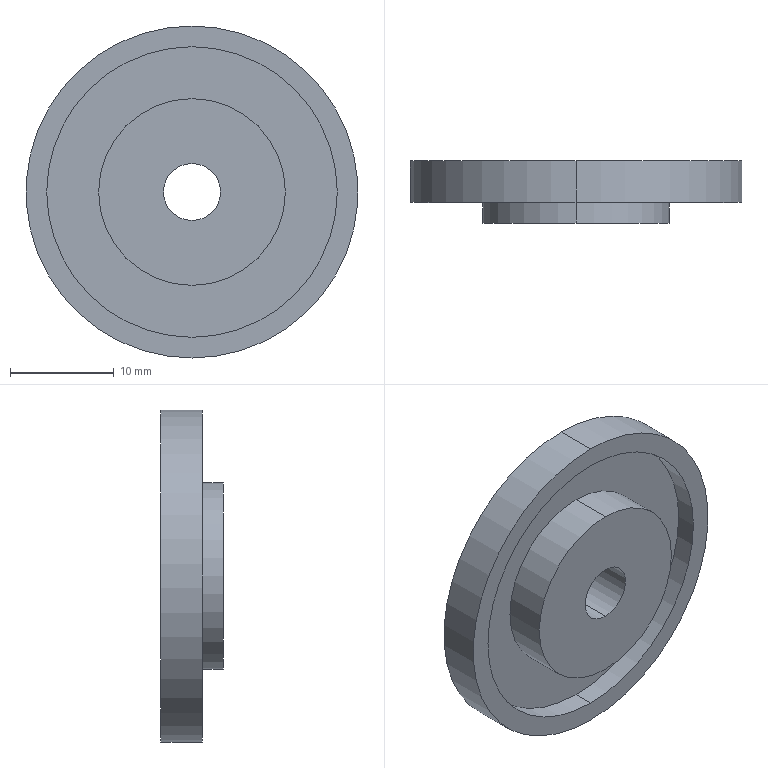Part | SolidWorks | features Revolution 1 | 1 solid | 14 faces | box 32 x 6 x 32 mm | volume 2776 mm3 | cylinder 8 | plane 4 | cone 2 | commonest cylinder face diameters 5.5 x2 18 x2 28 x2 32 x2
STEP:
#1=CARTESIAN_POINT('',(0.,-0.2262,-14.));
#2=VERTEX_POINT('',#1);
#3=CARTESIAN_POINT('',(0.,-0.2262,14.));
#4=VERTEX_POINT('',#3);
#5=CARTESIAN_POINT('',(0.,-0.2262,0.));
#6=DIRECTION('',(0.,1.,0.));
#7=DIRECTION('',(0.,0.,1.));
#8=AXIS2_PLACEMENT_3D('',#5,#6,#7);
#9=CIRCLE('',#8,14.);
#10=EDGE_CURVE('',#2,#4,#9,.T.);
#11=ORIENTED_EDGE('',*,*,#10,.F.);
#12=CARTESIAN_POINT('',(0.,1.774,-14.));
#13=VERTEX_POINT('',#12);
#14=CARTESIAN_POINT('',(0.,9.909,-14.));
#15=DIRECTION('',(0.,1.,0.));
#16=VECTOR('',#15,1000.);
#17=LINE('',#14,#16);
#18=EDGE_CURVE('',#2,#13,#17,.T.);
#19=ORIENTED_EDGE('',*,*,#18,.T.);
#20=CARTESIAN_POINT('',(0.,1.774,14.));
#21=VERTEX_POINT('',#20);
#22=CARTESIAN_POINT('',(0.,1.774,0.));
#23=DIRECTION('',(0.,1.,0.));
#24=DIRECTION('',(0.,0.,1.));
#25=AXIS2_PLACEMENT_3D('',#22,#23,#24);
#26=CIRCLE('',#25,14.);
#27=EDGE_CURVE('',#13,#21,#26,.T.);
#28=ORIENTED_EDGE('',*,*,#27,.T.);
#29=CARTESIAN_POINT('',(0.,9.909,14.));
#30=DIRECTION('',(0.,1.,0.));
#31=VECTOR('',#30,1000.);
#32=LINE('',#29,#31);
#33=EDGE_CURVE('',#4,#21,#32,.T.);
#34=ORIENTED_EDGE('',*,*,#33,.F.);
#35=EDGE_LOOP('',(#11,#19,#28,#34));
#36=FACE_OUTER_BOUND('',#35,.T.);
#37=CARTESIAN_POINT('',(0.,9.909,0.));
#38=DIRECTION('',(0.,1.,0.));
#39=DIRECTION('',(0.,0.,1.));
#40=AXIS2_PLACEMENT_3D('',#37,#38,#39);
#41=CYLINDRICAL_SURFACE('',#40,14.);
#42=ADVANCED_FACE('',(#36),#41,.F.);
#43=CARTESIAN_POINT('',(0.,-0.2262,16.));
#44=VERTEX_POINT('',#43);
#45=CARTESIAN_POINT('',(0.,-0.2262,-16.));
#46=VERTEX_POINT('',#45);
#47=CARTESIAN_POINT('',(0.,-0.2262,0.));
#48=DIRECTION('',(0.,1.,0.));
#49=DIRECTION('',(0.,0.,1.));
#50=AXIS2_PLACEMENT_3D('',#47,#48,#49);
#51=CIRCLE('',#50,16.);
#52=EDGE_CURVE('',#44,#46,#51,.T.);
#53=ORIENTED_EDGE('',*,*,#52,.T.);
#54=CARTESIAN_POINT('',(0.,3.774,-16.));
#55=VERTEX_POINT('',#54);
#56=CARTESIAN_POINT('',(0.,9.909,-16.));
#57=DIRECTION('',(0.,1.,0.));
#58=VECTOR('',#57,1000.);
#59=LINE('',#56,#58);
#60=EDGE_CURVE('',#46,#55,#59,.T.);
#61=ORIENTED_EDGE('',*,*,#60,.T.);
#62=CARTESIAN_POINT('',(0.,3.774,16.));
#63=VERTEX_POINT('',#62);
#64=CARTESIAN_POINT('',(0.,3.774,0.));
#65=DIRECTION('',(0.,1.,0.));
#66=DIRECTION('',(0.,0.,1.));
#67=AXIS2_PLACEMENT_3D('',#64,#65,#66);
#68=CIRCLE('',#67,16.);
#69=EDGE_CURVE('',#63,#55,#68,.T.);
#70=ORIENTED_EDGE('',*,*,#69,.F.);
#71=CARTESIAN_POINT('',(0.,9.909,16.));
#72=DIRECTION('',(0.,1.,0.));
#73=VECTOR('',#72,1000.);
#74=LINE('',#71,#73);
#75=EDGE_CURVE('',#44,#63,#74,.T.);
#76=ORIENTED_EDGE('',*,*,#75,.F.);
#77=EDGE_LOOP('',(#53,#61,#70,#76));
#78=FACE_OUTER_BOUND('',#77,.T.);
#79=CARTESIAN_POINT('',(0.,9.909,0.));
#80=DIRECTION('',(0.,1.,0.));
#81=DIRECTION('',(0.,0.,1.));
#82=AXIS2_PLACEMENT_3D('',#79,#80,#81);
#83=CYLINDRICAL_SURFACE('',#82,16.);
#84=ADVANCED_FACE('',(#78),#83,.T.);
#85=CARTESIAN_POINT('',(0.,1.774,-2.75));
#86=VERTEX_POINT('',#85);
#87=CARTESIAN_POINT('',(0.,1.774,2.75));
#88=VERTEX_POINT('',#87);
#89=CARTESIAN_POINT('',(0.,1.774,0.));
#90=DIRECTION('',(0.,1.,0.));
#91=DIRECTION('',(0.,0.,1.));
#92=AXIS2_PLACEMENT_3D('',#89,#90,#91);
#93=CIRCLE('',#92,2.75);
#94=EDGE_CURVE('',#86,#88,#93,.T.);
#95=ORIENTED_EDGE('',*,*,#94,.F.);
#96=CARTESIAN_POINT('',(0.,3.774,-6.214));
#97=VERTEX_POINT('',#96);
#98=CARTESIAN_POINT('',(0.,1.774,-2.75));
#99=DIRECTION('',(0.,0.5,-0.866));
#100=VECTOR('',#99,1000.);
#101=LINE('',#98,#100);
#102=EDGE_CURVE('',#86,#97,#101,.T.);
#103=ORIENTED_EDGE('',*,*,#102,.T.);
#104=CARTESIAN_POINT('',(0.,3.774,6.214));
#105=VERTEX_POINT('',#104);
#106=CARTESIAN_POINT('',(0.,3.774,0.));
#107=DIRECTION('',(0.,1.,0.));
#108=DIRECTION('',(0.,0.,1.));
#109=AXIS2_PLACEMENT_3D('',#106,#107,#108);
#110=CIRCLE('',#109,6.214);
#111=EDGE_CURVE('',#97,#105,#110,.T.);
#112=ORIENTED_EDGE('',*,*,#111,.T.);
#113=CARTESIAN_POINT('',(0.,1.774,2.75));
#114=DIRECTION('',(0.,0.5,0.866));
#115=VECTOR('',#114,1000.);
#116=LINE('',#113,#115);
#117=EDGE_CURVE('',#88,#105,#116,.T.);
#118=ORIENTED_EDGE('',*,*,#117,.F.);
#119=EDGE_LOOP('',(#95,#103,#112,#118));
#120=FACE_OUTER_BOUND('',#119,.T.);
#121=CARTESIAN_POINT('',(0.,1.774,0.));
#122=DIRECTION('',(0.,1.,0.));
#123=DIRECTION('',(0.,0.,1.));
#124=AXIS2_PLACEMENT_3D('',#121,#122,#123);
#125=CONICAL_SURFACE('',#124,2.75,1.047);
#126=ADVANCED_FACE('',(#120),#125,.F.);
#127=CARTESIAN_POINT('',(0.,-2.226,-2.75));
#128=VERTEX_POINT('',#127);
#129=CARTESIAN_POINT('',(0.,-2.226,2.75));
#130=VERTEX_POINT('',#129);
#131=CARTESIAN_POINT('',(0.,-2.226,0.));
#132=DIRECTION('',(0.,1.,0.));
#133=DIRECTION('',(0.,0.,1.));
#134=AXIS2_PLACEMENT_3D('',#131,#132,#133);
#135=CIRCLE('',#134,2.75);
#136=EDGE_CURVE('',#128,#130,#135,.T.);
#137=ORIENTED_EDGE('',*,*,#136,.F.);
#138=CARTESIAN_POINT('',(0.,9.909,-2.75));
#139=DIRECTION('',(0.,1.,0.));
#140=VECTOR('',#139,1000.);
#141=LINE('',#138,#140);
#142=EDGE_CURVE('',#128,#86,#141,.T.);
#143=ORIENTED_EDGE('',*,*,#142,.T.);
#144=ORIENTED_EDGE('',*,*,#94,.T.);
#145=CARTESIAN_POINT('',(0.,9.909,2.75));
#146=DIRECTION('',(0.,1.,0.));
#147=VECTOR('',#146,1000.);
#148=LINE('',#145,#147);
#149=EDGE_CURVE('',#130,#88,#148,.T.);
#150=ORIENTED_EDGE('',*,*,#149,.F.);
#151=EDGE_LOOP('',(#137,#143,#144,#150));
#152=FACE_OUTER_BOUND('',#151,.T.);
#153=CARTESIAN_POINT('',(0.,9.909,0.));
#154=DIRECTION('',(0.,1.,0.));
#155=DIRECTION('',(0.,0.,1.));
#156=AXIS2_PLACEMENT_3D('',#153,#154,#155);
#157=CYLINDRICAL_SURFACE('',#156,2.75);
#158=ADVANCED_FACE('',(#152),#157,.F.);
#159=CARTESIAN_POINT('',(0.,-2.226,9.));
#160=VERTEX_POINT('',#159);
#161=CARTESIAN_POINT('',(0.,-2.226,-9.));
#162=VERTEX_POINT('',#161);
#163=CARTESIAN_POINT('',(0.,-2.226,0.));
#164=DIRECTION('',(0.,1.,0.));
#165=DIRECTION('',(0.,0.,1.));
#166=AXIS2_PLACEMENT_3D('',#163,#164,#165);
#167=CIRCLE('',#166,9.);
#168=EDGE_CURVE('',#160,#162,#167,.T.);
#169=ORIENTED_EDGE('',*,*,#168,.T.);
#170=CARTESIAN_POINT('',(0.,1.774,-9.));
#171=VERTEX_POINT('',#170);
#172=CARTESIAN_POINT('',(0.,9.909,-9.));
#173=DIRECTION('',(0.,1.,0.));
#174=VECTOR('',#173,1000.);
#175=LINE('',#172,#174);
#176=EDGE_CURVE('',#162,#171,#175,.T.);
#177=ORIENTED_EDGE('',*,*,#176,.T.);
#178=CARTESIAN_POINT('',(0.,1.774,9.));
#179=VERTEX_POINT('',#178);
#180=CARTESIAN_POINT('',(0.,1.774,0.));
#181=DIRECTION('',(0.,1.,0.));
#182=DIRECTION('',(0.,0.,1.));
#183=AXIS2_PLACEMENT_3D('',#180,#181,#182);
#184=CIRCLE('',#183,9.);
#185=EDGE_CURVE('',#179,#171,#184,.T.);
#186=ORIENTED_EDGE('',*,*,#185,.F.);
#187=CARTESIAN_POINT('',(0.,9.909,9.));
#188=DIRECTION('',(0.,1.,0.));
#189=VECTOR('',#188,1000.);
#190=LINE('',#187,#189);
#191=EDGE_CURVE('',#160,#179,#190,.T.);
#192=ORIENTED_EDGE('',*,*,#191,.F.);
#193=EDGE_LOOP('',(#169,#177,#186,#192));
#194=FACE_OUTER_BOUND('',#193,.T.);
#195=CARTESIAN_POINT('',(0.,9.909,0.));
#196=DIRECTION('',(0.,1.,0.));
#197=DIRECTION('',(0.,0.,1.));
#198=AXIS2_PLACEMENT_3D('',#195,#196,#197);
#199=CYLINDRICAL_SURFACE('',#198,9.);
#200=ADVANCED_FACE('',(#194),#199,.T.);
#201=ORIENTED_EDGE('',*,*,#176,.F.);
#202=CARTESIAN_POINT('',(0.,-2.226,0.));
#203=DIRECTION('',(0.,1.,0.));
#204=DIRECTION('',(0.,0.,1.));
#205=AXIS2_PLACEMENT_3D('',#202,#203,#204);
#206=CIRCLE('',#205,9.);
#207=EDGE_CURVE('',#162,#160,#206,.T.);
#208=ORIENTED_EDGE('',*,*,#207,.T.);
#209=ORIENTED_EDGE('',*,*,#191,.T.);
#210=CARTESIAN_POINT('',(0.,1.774,0.));
#211=DIRECTION('',(0.,1.,0.));
#212=DIRECTION('',(0.,0.,1.));
#213=AXIS2_PLACEMENT_3D('',#210,#211,#212);
#214=CIRCLE('',#213,9.);
#215=EDGE_CURVE('',#171,#179,#214,.T.);
#216=ORIENTED_EDGE('',*,*,#215,.F.);
#217=EDGE_LOOP('',(#201,#208,#209,#216));
#218=FACE_OUTER_BOUND('',#217,.T.);
#219=CARTESIAN_POINT('',(0.,9.909,0.));
#220=DIRECTION('',(0.,1.,0.));
#221=DIRECTION('',(0.,0.,1.));
#222=AXIS2_PLACEMENT_3D('',#219,#220,#221);
#223=CYLINDRICAL_SURFACE('',#222,9.);
#224=ADVANCED_FACE('',(#218),#223,.T.);
#225=CARTESIAN_POINT('',(0.,-2.226,0.));
#226=DIRECTION('',(0.,1.,0.));
#227=DIRECTION('',(0.,0.,1.));
#228=AXIS2_PLACEMENT_3D('',#225,#226,#227);
#229=CIRCLE('',#228,2.75);
#230=EDGE_CURVE('',#130,#128,#229,.T.);
#231=ORIENTED_EDGE('',*,*,#230,.T.);
#232=ORIENTED_EDGE('',*,*,#136,.T.);
#233=EDGE_LOOP('',(#231,#232));
#234=FACE_BOUND('',#233,.T.);
#235=ORIENTED_EDGE('',*,*,#168,.F.);
#236=ORIENTED_EDGE('',*,*,#207,.F.);
#237=EDGE_LOOP('',(#235,#236));
#238=FACE_OUTER_BOUND('',#237,.T.);
#239=CARTESIAN_POINT('',(-2.75,-2.226,0.));
#240=DIRECTION('',(0.,-1.,0.));
#241=DIRECTION('',(0.,0.,-1.));
#242=AXIS2_PLACEMENT_3D('',#239,#240,#241);
#243=PLANE('',#242);
#244=ADVANCED_FACE('',(#234,#238),#243,.T.);
#245=ORIENTED_EDGE('',*,*,#142,.F.);
#246=ORIENTED_EDGE('',*,*,#230,.F.);
#247=ORIENTED_EDGE('',*,*,#149,.T.);
#248=CARTESIAN_POINT('',(0.,1.774,0.));
#249=DIRECTION('',(0.,1.,0.));
#250=DIRECTION('',(0.,0.,1.));
#251=AXIS2_PLACEMENT_3D('',#248,#249,#250);
#252=CIRCLE('',#251,2.75);
#253=EDGE_CURVE('',#88,#86,#252,.T.);
#254=ORIENTED_EDGE('',*,*,#253,.T.);
#255=EDGE_LOOP('',(#245,#246,#247,#254));
#256=FACE_OUTER_BOUND('',#255,.T.);
#257=CARTESIAN_POINT('',(0.,9.909,0.));
#258=DIRECTION('',(0.,1.,0.));
#259=DIRECTION('',(0.,0.,1.));
#260=AXIS2_PLACEMENT_3D('',#257,#258,#259);
#261=CYLINDRICAL_SURFACE('',#260,2.75);
#262=ADVANCED_FACE('',(#256),#261,.F.);
#263=ORIENTED_EDGE('',*,*,#102,.F.);
#264=ORIENTED_EDGE('',*,*,#253,.F.);
#265=ORIENTED_EDGE('',*,*,#117,.T.);
#266=CARTESIAN_POINT('',(0.,3.774,0.));
#267=DIRECTION('',(0.,1.,0.));
#268=DIRECTION('',(0.,0.,1.));
#269=AXIS2_PLACEMENT_3D('',#266,#267,#268);
#270=CIRCLE('',#269,6.214);
#271=EDGE_CURVE('',#105,#97,#270,.T.);
#272=ORIENTED_EDGE('',*,*,#271,.T.);
#273=EDGE_LOOP('',(#263,#264,#265,#272));
#274=FACE_OUTER_BOUND('',#273,.T.);
#275=CARTESIAN_POINT('',(0.,1.774,0.));
#276=DIRECTION('',(0.,1.,0.));
#277=DIRECTION('',(0.,0.,1.));
#278=AXIS2_PLACEMENT_3D('',#275,#276,#277);
#279=CONICAL_SURFACE('',#278,2.75,1.047);
#280=ADVANCED_FACE('',(#274),#279,.F.);
#281=ORIENTED_EDGE('',*,*,#69,.T.);
#282=CARTESIAN_POINT('',(0.,3.774,0.));
#283=DIRECTION('',(0.,1.,0.));
#284=DIRECTION('',(0.,0.,1.));
#285=AXIS2_PLACEMENT_3D('',#282,#283,#284);
#286=CIRCLE('',#285,16.);
#287=EDGE_CURVE('',#55,#63,#286,.T.);
#288=ORIENTED_EDGE('',*,*,#287,.T.);
#289=EDGE_LOOP('',(#281,#288));
#290=FACE_OUTER_BOUND('',#289,.T.);
#291=ORIENTED_EDGE('',*,*,#271,.F.);
#292=ORIENTED_EDGE('',*,*,#111,.F.);
#293=EDGE_LOOP('',(#291,#292));
#294=FACE_BOUND('',#293,.T.);
#295=CARTESIAN_POINT('',(-16.,3.774,0.));
#296=DIRECTION('',(0.,1.,0.));
#297=DIRECTION('',(0.,0.,1.));
#298=AXIS2_PLACEMENT_3D('',#295,#296,#297);
#299=PLANE('',#298);
#300=ADVANCED_FACE('',(#290,#294),#299,.T.);
#301=ORIENTED_EDGE('',*,*,#60,.F.);
#302=CARTESIAN_POINT('',(0.,-0.2262,0.));
#303=DIRECTION('',(0.,1.,0.));
#304=DIRECTION('',(0.,0.,1.));
#305=AXIS2_PLACEMENT_3D('',#302,#303,#304);
#306=CIRCLE('',#305,16.);
#307=EDGE_CURVE('',#46,#44,#306,.T.);
#308=ORIENTED_EDGE('',*,*,#307,.T.);
#309=ORIENTED_EDGE('',*,*,#75,.T.);
#310=ORIENTED_EDGE('',*,*,#287,.F.);
#311=EDGE_LOOP('',(#301,#308,#309,#310));
#312=FACE_OUTER_BOUND('',#311,.T.);
#313=CARTESIAN_POINT('',(0.,9.909,0.));
#314=DIRECTION('',(0.,1.,0.));
#315=DIRECTION('',(0.,0.,1.));
#316=AXIS2_PLACEMENT_3D('',#313,#314,#315);
#317=CYLINDRICAL_SURFACE('',#316,16.);
#318=ADVANCED_FACE('',(#312),#317,.T.);
#319=CARTESIAN_POINT('',(0.,-0.2262,0.));
#320=DIRECTION('',(0.,1.,0.));
#321=DIRECTION('',(0.,0.,1.));
#322=AXIS2_PLACEMENT_3D('',#319,#320,#321);
#323=CIRCLE('',#322,14.);
#324=EDGE_CURVE('',#4,#2,#323,.T.);
#325=ORIENTED_EDGE('',*,*,#324,.T.);
#326=ORIENTED_EDGE('',*,*,#10,.T.);
#327=EDGE_LOOP('',(#325,#326));
#328=FACE_BOUND('',#327,.T.);
#329=ORIENTED_EDGE('',*,*,#52,.F.);
#330=ORIENTED_EDGE('',*,*,#307,.F.);
#331=EDGE_LOOP('',(#329,#330));
#332=FACE_OUTER_BOUND('',#331,.T.);
#333=CARTESIAN_POINT('',(-14.,-0.2262,0.));
#334=DIRECTION('',(0.,-1.,0.));
#335=DIRECTION('',(0.,0.,-1.));
#336=AXIS2_PLACEMENT_3D('',#333,#334,#335);
#337=PLANE('',#336);
#338=ADVANCED_FACE('',(#328,#332),#337,.T.);
#339=ORIENTED_EDGE('',*,*,#18,.F.);
#340=ORIENTED_EDGE('',*,*,#324,.F.);
#341=ORIENTED_EDGE('',*,*,#33,.T.);
#342=CARTESIAN_POINT('',(0.,1.774,0.));
#343=DIRECTION('',(0.,1.,0.));
#344=DIRECTION('',(0.,0.,1.));
#345=AXIS2_PLACEMENT_3D('',#342,#343,#344);
#346=CIRCLE('',#345,14.);
#347=EDGE_CURVE('',#21,#13,#346,.T.);
#348=ORIENTED_EDGE('',*,*,#347,.T.);
#349=EDGE_LOOP('',(#339,#340,#341,#348));
#350=FACE_OUTER_BOUND('',#349,.T.);
#351=CARTESIAN_POINT('',(0.,9.909,0.));
#352=DIRECTION('',(0.,1.,0.));
#353=DIRECTION('',(0.,0.,1.));
#354=AXIS2_PLACEMENT_3D('',#351,#352,#353);
#355=CYLINDRICAL_SURFACE('',#354,14.);
#356=ADVANCED_FACE('',(#350),#355,.F.);
#357=ORIENTED_EDGE('',*,*,#185,.T.);
#358=ORIENTED_EDGE('',*,*,#215,.T.);
#359=EDGE_LOOP('',(#357,#358));
#360=FACE_BOUND('',#359,.T.);
#361=ORIENTED_EDGE('',*,*,#347,.F.);
#362=ORIENTED_EDGE('',*,*,#27,.F.);
#363=EDGE_LOOP('',(#361,#362));
#364=FACE_OUTER_BOUND('',#363,.T.);
#365=CARTESIAN_POINT('',(-9.,1.774,0.));
#366=DIRECTION('',(0.,-1.,0.));
#367=DIRECTION('',(0.,0.,-1.));
#368=AXIS2_PLACEMENT_3D('',#365,#366,#367);
#369=PLANE('',#368);
#370=ADVANCED_FACE('',(#360,#364),#369,.T.);
#371=CLOSED_SHELL('',(#42,#84,#126,#158,#200,#224,#244,#262,#280,#300,#318,#338,#356,#370));
#372=MANIFOLD_SOLID_BREP('',#371);
#373=CARTESIAN_POINT('',(0.,0.,0.));
#374=DIRECTION('',(0.,0.,1.));
#375=DIRECTION('',(1.,0.,0.));
#376=AXIS2_PLACEMENT_3D('',#373,#374,#375);
#377=(LENGTH_UNIT()NAMED_UNIT(*)SI_UNIT(.MILLI.,.METRE.));
#378=UNCERTAINTY_MEASURE_WITH_UNIT(LENGTH_MEASURE(0.00001),#377,'','');
#379=(NAMED_UNIT(*)PLANE_ANGLE_UNIT()SI_UNIT($,.RADIAN.));
#380=(NAMED_UNIT(*)SI_UNIT($,.STERADIAN.)SOLID_ANGLE_UNIT());
#381=(GEOMETRIC_REPRESENTATION_CONTEXT(3)GLOBAL_UNCERTAINTY_ASSIGNED_CONTEXT((#378))GLOBAL_UNIT_ASSIGNED_CONTEXT((#377,#379,#380))REPRESENTATION_CONTEXT('',''));
#382=ADVANCED_BREP_SHAPE_REPRESENTATION('',(#372,#376),#381);